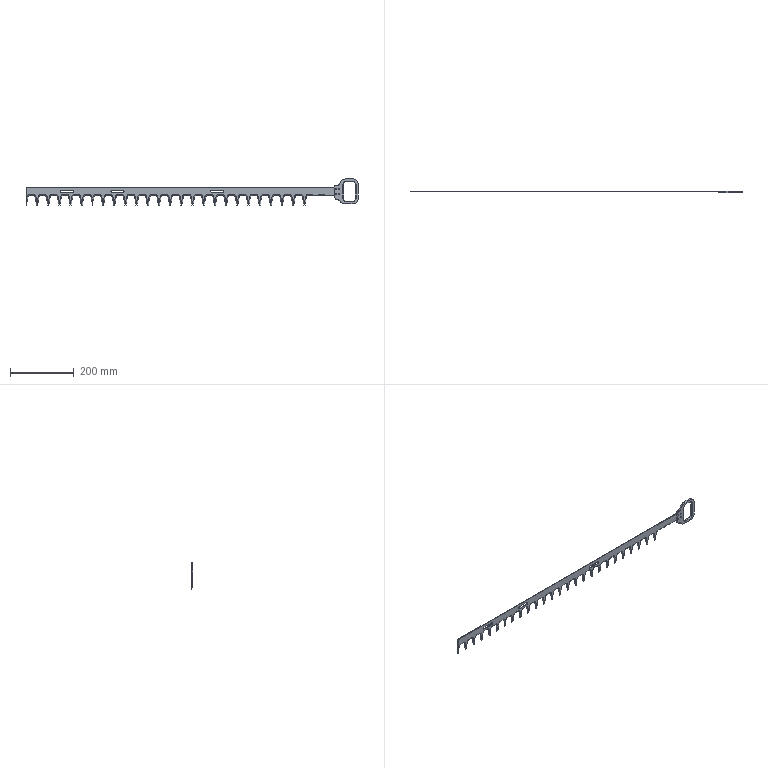Part | SolidWorks | 6 solids | 345 faces | box 1039 x 6.076 x 81.5 mm | volume 84065 mm3 | plane 201 | cone 78 | cylinder 66 | commonest cylinder face diameters 0.4 x16 2.5 x8 3 x8 3.4 x8 5.36 x8 8 x6